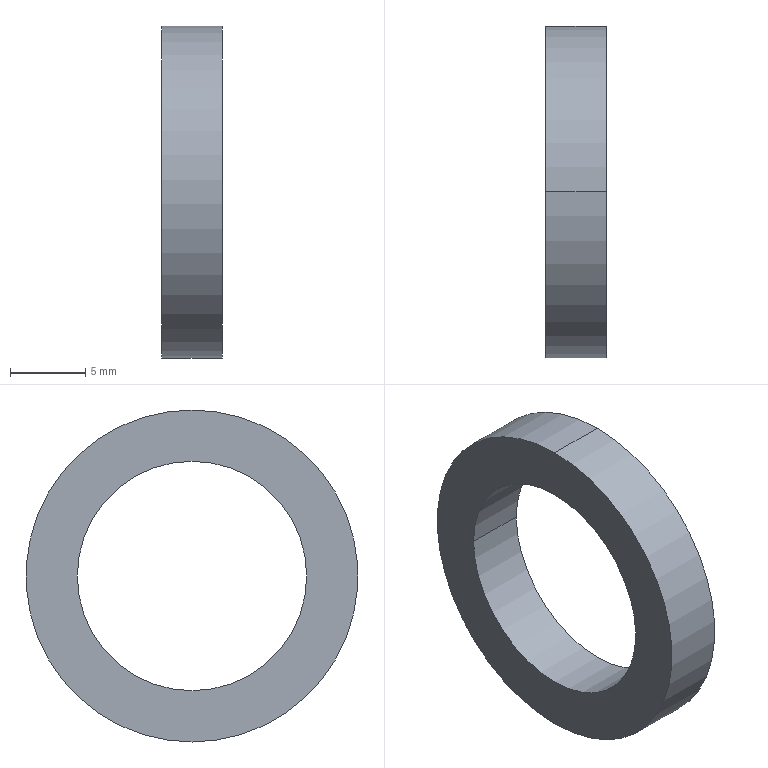Part | NX | 1 solid | 6 faces | box 4 x 22 x 22 mm | volume 794.697 mm3 | cylinder 4 | plane 2 | commonest cylinder face diameters 15.2 x2 22 x2
STEP:
#1=CARTESIAN_POINT('',(-140.,161.,-68.));
#2=VERTEX_POINT('',#1);
#3=CARTESIAN_POINT('',(-140.,161.,-46.));
#4=VERTEX_POINT('',#3);
#5=CARTESIAN_POINT('',(-140.,161.,-57.));
#6=DIRECTION('',(-1.,0.,0.));
#7=DIRECTION('',(0.,0.,1.));
#8=AXIS2_PLACEMENT_3D('',#5,#6,#7);
#9=CIRCLE('',#8,11.);
#10=EDGE_CURVE('',#2,#4,#9,.T.);
#11=ORIENTED_EDGE('',*,*,#10,.T.);
#12=CARTESIAN_POINT('',(-144.,161.,-46.));
#13=VERTEX_POINT('',#12);
#14=CARTESIAN_POINT('',(-144.,161.,-46.));
#15=DIRECTION('',(-1.,0.,0.));
#16=VECTOR('',#15,1000.);
#17=LINE('',#14,#16);
#18=EDGE_CURVE('',#13,#4,#17,.F.);
#19=ORIENTED_EDGE('',*,*,#18,.F.);
#20=CARTESIAN_POINT('',(-144.,161.,-68.));
#21=VERTEX_POINT('',#20);
#22=CARTESIAN_POINT('',(-144.,161.,-57.));
#23=DIRECTION('',(-1.,0.,0.));
#24=DIRECTION('',(0.,0.,1.));
#25=AXIS2_PLACEMENT_3D('',#22,#23,#24);
#26=CIRCLE('',#25,11.);
#27=EDGE_CURVE('',#21,#13,#26,.T.);
#28=ORIENTED_EDGE('',*,*,#27,.F.);
#29=CARTESIAN_POINT('',(-144.,161.,-68.));
#30=DIRECTION('',(-1.,0.,0.));
#31=VECTOR('',#30,1000.);
#32=LINE('',#29,#31);
#33=EDGE_CURVE('',#21,#2,#32,.F.);
#34=ORIENTED_EDGE('',*,*,#33,.T.);
#35=EDGE_LOOP('',(#11,#19,#28,#34));
#36=FACE_BOUND('',#35,.T.);
#37=CARTESIAN_POINT('',(-144.,161.,-57.));
#38=DIRECTION('',(-1.,0.,0.));
#39=DIRECTION('',(0.,0.,1.));
#40=AXIS2_PLACEMENT_3D('',#37,#38,#39);
#41=CYLINDRICAL_SURFACE('',#40,11.);
#42=ADVANCED_FACE('',(#36),#41,.T.);
#43=ORIENTED_EDGE('',*,*,#33,.F.);
#44=CARTESIAN_POINT('',(-144.,161.,-57.));
#45=DIRECTION('',(-1.,0.,0.));
#46=DIRECTION('',(0.,0.,1.));
#47=AXIS2_PLACEMENT_3D('',#44,#45,#46);
#48=CIRCLE('',#47,11.);
#49=EDGE_CURVE('',#13,#21,#48,.T.);
#50=ORIENTED_EDGE('',*,*,#49,.F.);
#51=ORIENTED_EDGE('',*,*,#18,.T.);
#52=CARTESIAN_POINT('',(-140.,161.,-57.));
#53=DIRECTION('',(-1.,0.,0.));
#54=DIRECTION('',(0.,0.,1.));
#55=AXIS2_PLACEMENT_3D('',#52,#53,#54);
#56=CIRCLE('',#55,11.);
#57=EDGE_CURVE('',#4,#2,#56,.T.);
#58=ORIENTED_EDGE('',*,*,#57,.T.);
#59=EDGE_LOOP('',(#43,#50,#51,#58));
#60=FACE_BOUND('',#59,.T.);
#61=CARTESIAN_POINT('',(-144.,161.,-57.));
#62=DIRECTION('',(-1.,0.,0.));
#63=DIRECTION('',(0.,0.,1.));
#64=AXIS2_PLACEMENT_3D('',#61,#62,#63);
#65=CYLINDRICAL_SURFACE('',#64,11.);
#66=ADVANCED_FACE('',(#60),#65,.T.);
#67=CARTESIAN_POINT('',(-140.,168.6,-57.));
#68=VERTEX_POINT('',#67);
#69=CARTESIAN_POINT('',(-140.,153.4,-57.));
#70=VERTEX_POINT('',#69);
#71=CARTESIAN_POINT('',(-140.,161.,-57.));
#72=DIRECTION('',(-1.,0.,0.));
#73=DIRECTION('',(0.,-1.,0.));
#74=AXIS2_PLACEMENT_3D('',#71,#72,#73);
#75=CIRCLE('',#74,7.6);
#76=EDGE_CURVE('',#68,#70,#75,.T.);
#77=ORIENTED_EDGE('',*,*,#76,.F.);
#78=CARTESIAN_POINT('',(-144.,168.6,-57.));
#79=VERTEX_POINT('',#78);
#80=CARTESIAN_POINT('',(-144.,168.6,-57.));
#81=DIRECTION('',(-1.,0.,0.));
#82=VECTOR('',#81,1000.);
#83=LINE('',#80,#82);
#84=EDGE_CURVE('',#79,#68,#83,.F.);
#85=ORIENTED_EDGE('',*,*,#84,.F.);
#86=CARTESIAN_POINT('',(-144.,153.4,-57.));
#87=VERTEX_POINT('',#86);
#88=CARTESIAN_POINT('',(-144.,161.,-57.));
#89=DIRECTION('',(-1.,0.,0.));
#90=DIRECTION('',(0.,-1.,0.));
#91=AXIS2_PLACEMENT_3D('',#88,#89,#90);
#92=CIRCLE('',#91,7.6);
#93=EDGE_CURVE('',#79,#87,#92,.T.);
#94=ORIENTED_EDGE('',*,*,#93,.T.);
#95=CARTESIAN_POINT('',(-144.,153.4,-57.));
#96=DIRECTION('',(-1.,0.,0.));
#97=VECTOR('',#96,1000.);
#98=LINE('',#95,#97);
#99=EDGE_CURVE('',#87,#70,#98,.F.);
#100=ORIENTED_EDGE('',*,*,#99,.T.);
#101=EDGE_LOOP('',(#77,#85,#94,#100));
#102=FACE_BOUND('',#101,.T.);
#103=CARTESIAN_POINT('',(-144.,161.,-57.));
#104=DIRECTION('',(-1.,0.,0.));
#105=DIRECTION('',(0.,-1.,0.));
#106=AXIS2_PLACEMENT_3D('',#103,#104,#105);
#107=CYLINDRICAL_SURFACE('',#106,7.6);
#108=ADVANCED_FACE('',(#102),#107,.F.);
#109=ORIENTED_EDGE('',*,*,#99,.F.);
#110=CARTESIAN_POINT('',(-144.,161.,-57.));
#111=DIRECTION('',(-1.,0.,0.));
#112=DIRECTION('',(0.,-1.,0.));
#113=AXIS2_PLACEMENT_3D('',#110,#111,#112);
#114=CIRCLE('',#113,7.6);
#115=EDGE_CURVE('',#87,#79,#114,.T.);
#116=ORIENTED_EDGE('',*,*,#115,.T.);
#117=ORIENTED_EDGE('',*,*,#84,.T.);
#118=CARTESIAN_POINT('',(-140.,161.,-57.));
#119=DIRECTION('',(-1.,0.,0.));
#120=DIRECTION('',(0.,-1.,0.));
#121=AXIS2_PLACEMENT_3D('',#118,#119,#120);
#122=CIRCLE('',#121,7.6);
#123=EDGE_CURVE('',#70,#68,#122,.T.);
#124=ORIENTED_EDGE('',*,*,#123,.F.);
#125=EDGE_LOOP('',(#109,#116,#117,#124));
#126=FACE_BOUND('',#125,.T.);
#127=CARTESIAN_POINT('',(-144.,161.,-57.));
#128=DIRECTION('',(-1.,0.,0.));
#129=DIRECTION('',(0.,-1.,0.));
#130=AXIS2_PLACEMENT_3D('',#127,#128,#129);
#131=CYLINDRICAL_SURFACE('',#130,7.6);
#132=ADVANCED_FACE('',(#126),#131,.F.);
#133=ORIENTED_EDGE('',*,*,#10,.F.);
#134=ORIENTED_EDGE('',*,*,#57,.F.);
#135=EDGE_LOOP('',(#133,#134));
#136=FACE_BOUND('',#135,.T.);
#137=ORIENTED_EDGE('',*,*,#76,.T.);
#138=ORIENTED_EDGE('',*,*,#123,.T.);
#139=EDGE_LOOP('',(#137,#138));
#140=FACE_BOUND('',#139,.T.);
#141=CARTESIAN_POINT('',(-140.,171.479,-46.149));
#142=DIRECTION('',(1.,0.,0.));
#143=DIRECTION('',(0.,-1.,0.));
#144=AXIS2_PLACEMENT_3D('',#141,#142,#143);
#145=PLANE('',#144);
#146=ADVANCED_FACE('',(#136,#140),#145,.T.);
#147=ORIENTED_EDGE('',*,*,#27,.T.);
#148=ORIENTED_EDGE('',*,*,#49,.T.);
#149=EDGE_LOOP('',(#147,#148));
#150=FACE_BOUND('',#149,.T.);
#151=ORIENTED_EDGE('',*,*,#93,.F.);
#152=ORIENTED_EDGE('',*,*,#115,.F.);
#153=EDGE_LOOP('',(#151,#152));
#154=FACE_BOUND('',#153,.T.);
#155=CARTESIAN_POINT('',(-144.,171.479,-46.149));
#156=DIRECTION('',(1.,0.,0.));
#157=DIRECTION('',(0.,-1.,0.));
#158=AXIS2_PLACEMENT_3D('',#155,#156,#157);
#159=PLANE('',#158);
#160=ADVANCED_FACE('',(#150,#154),#159,.F.);
#161=CLOSED_SHELL('',(#42,#66,#108,#132,#146,#160));
#162=MANIFOLD_SOLID_BREP('',#161);
#163=(LENGTH_UNIT()NAMED_UNIT(*)SI_UNIT(.MILLI.,.METRE.));
#164=UNCERTAINTY_MEASURE_WITH_UNIT(LENGTH_MEASURE(0.00001),#163,'','');
#165=(NAMED_UNIT(*)PLANE_ANGLE_UNIT()SI_UNIT($,.RADIAN.));
#166=(NAMED_UNIT(*)SI_UNIT($,.STERADIAN.)SOLID_ANGLE_UNIT());
#167=(GEOMETRIC_REPRESENTATION_CONTEXT(3)GLOBAL_UNCERTAINTY_ASSIGNED_CONTEXT((#164))GLOBAL_UNIT_ASSIGNED_CONTEXT((#163,#165,#166))REPRESENTATION_CONTEXT('',''));
#168=ADVANCED_BREP_SHAPE_REPRESENTATION('',(#162),#167);